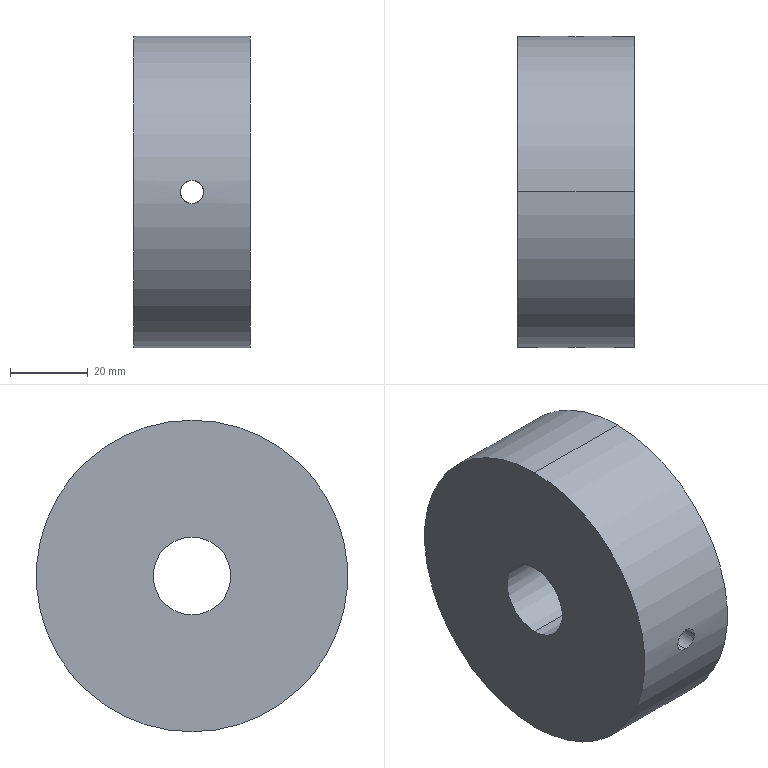Part | NX | features BREP 1 | 1 solid | 10 faces | box 30 x 80 x 80 mm | volume 139671 mm3 | cylinder 8 | plane 2 | commonest cylinder face diameters 6 x4 20 x2 80 x2
STEP:
#1=CARTESIAN_POINT('',(15.,39.887,-3.));
#2=VERTEX_POINT('',#1);
#3=CARTESIAN_POINT('',(15.,39.887,3.));
#4=VERTEX_POINT('',#3);
#5=CARTESIAN_POINT('',(15.,39.887,-3.));
#6=CARTESIAN_POINT('',(14.207,39.887,-3.));
#7=CARTESIAN_POINT('',(12.654,39.944,-2.35));
#8=CARTESIAN_POINT('',(11.674,40.028,-0.00292));
#9=CARTESIAN_POINT('',(12.651,39.944,2.349));
#10=CARTESIAN_POINT('',(14.207,39.887,3.));
#11=CARTESIAN_POINT('',(15.,39.887,3.));
#12=B_SPLINE_CURVE_WITH_KNOTS('',3,(#5,#6,#7,#8,#9,#10,#11),.UNSPECIFIED.,.F.,.F.,(4,1,1,1,4),(0.,0.002345,0.00469,0.007035,0.009381),.UNSPECIFIED.);
#13=EDGE_CURVE('',#2,#4,#12,.T.);
#14=ORIENTED_EDGE('',*,*,#13,.T.);
#15=CARTESIAN_POINT('',(15.,9.539,3.));
#16=VERTEX_POINT('',#15);
#17=CARTESIAN_POINT('',(15.,40.,3.));
#18=DIRECTION('',(0.,-1.,0.));
#19=VECTOR('',#18,1000.);
#20=LINE('',#17,#19);
#21=EDGE_CURVE('',#16,#4,#20,.F.);
#22=ORIENTED_EDGE('',*,*,#21,.F.);
#23=CARTESIAN_POINT('',(15.,9.539,-3.));
#24=VERTEX_POINT('',#23);
#25=CARTESIAN_POINT('',(15.,9.539,-3.));
#26=CARTESIAN_POINT('',(14.202,9.539,-3.));
#27=CARTESIAN_POINT('',(12.656,9.775,-2.35));
#28=CARTESIAN_POINT('',(11.672,10.112,-0.004774));
#29=CARTESIAN_POINT('',(12.655,9.775,2.351));
#30=CARTESIAN_POINT('',(14.202,9.539,3.));
#31=CARTESIAN_POINT('',(15.,9.539,3.));
#32=B_SPLINE_CURVE_WITH_KNOTS('',3,(#25,#26,#27,#28,#29,#30,#31),.UNSPECIFIED.,.F.,.F.,(4,1,1,1,4),(0.,0.002358,0.004715,0.007073,0.009431),.UNSPECIFIED.);
#33=EDGE_CURVE('',#24,#16,#32,.T.);
#34=ORIENTED_EDGE('',*,*,#33,.F.);
#35=CARTESIAN_POINT('',(15.,40.,-3.));
#36=DIRECTION('',(0.,-1.,0.));
#37=VECTOR('',#36,1000.);
#38=LINE('',#35,#37);
#39=EDGE_CURVE('',#24,#2,#38,.F.);
#40=ORIENTED_EDGE('',*,*,#39,.T.);
#41=EDGE_LOOP('',(#14,#22,#34,#40));
#42=FACE_BOUND('',#41,.T.);
#43=CARTESIAN_POINT('',(15.,40.,0.));
#44=DIRECTION('',(0.,-1.,0.));
#45=DIRECTION('',(0.,0.,1.));
#46=AXIS2_PLACEMENT_3D('',#43,#44,#45);
#47=CYLINDRICAL_SURFACE('',#46,3.);
#48=ADVANCED_FACE('',(#42),#47,.F.);
#49=CARTESIAN_POINT('',(15.,-9.539,3.));
#50=VERTEX_POINT('',#49);
#51=CARTESIAN_POINT('',(15.,-9.539,-3.));
#52=VERTEX_POINT('',#51);
#53=CARTESIAN_POINT('',(15.,-9.539,3.));
#54=CARTESIAN_POINT('',(14.202,-9.539,3.));
#55=CARTESIAN_POINT('',(12.656,-9.775,2.35));
#56=CARTESIAN_POINT('',(11.672,-10.112,0.004774));
#57=CARTESIAN_POINT('',(12.655,-9.775,-2.351));
#58=CARTESIAN_POINT('',(14.202,-9.539,-3.));
#59=CARTESIAN_POINT('',(15.,-9.539,-3.));
#60=B_SPLINE_CURVE_WITH_KNOTS('',3,(#53,#54,#55,#56,#57,#58,#59),.UNSPECIFIED.,.F.,.F.,(4,1,1,1,4),(0.,0.002358,0.004715,0.007073,0.009431),.UNSPECIFIED.);
#61=EDGE_CURVE('',#50,#52,#60,.T.);
#62=ORIENTED_EDGE('',*,*,#61,.F.);
#63=CARTESIAN_POINT('',(15.,-39.887,3.));
#64=VERTEX_POINT('',#63);
#65=CARTESIAN_POINT('',(15.,40.,3.));
#66=DIRECTION('',(0.,-1.,0.));
#67=VECTOR('',#66,1000.);
#68=LINE('',#65,#67);
#69=EDGE_CURVE('',#64,#50,#68,.F.);
#70=ORIENTED_EDGE('',*,*,#69,.F.);
#71=CARTESIAN_POINT('',(15.,-39.887,-3.));
#72=VERTEX_POINT('',#71);
#73=CARTESIAN_POINT('',(15.,-39.887,3.));
#74=CARTESIAN_POINT('',(14.207,-39.887,3.));
#75=CARTESIAN_POINT('',(12.654,-39.944,2.35));
#76=CARTESIAN_POINT('',(11.674,-40.028,0.00292));
#77=CARTESIAN_POINT('',(12.651,-39.944,-2.349));
#78=CARTESIAN_POINT('',(14.207,-39.887,-3.));
#79=CARTESIAN_POINT('',(15.,-39.887,-3.));
#80=B_SPLINE_CURVE_WITH_KNOTS('',3,(#73,#74,#75,#76,#77,#78,#79),.UNSPECIFIED.,.F.,.F.,(4,1,1,1,4),(0.,0.002345,0.00469,0.007035,0.009381),.UNSPECIFIED.);
#81=EDGE_CURVE('',#64,#72,#80,.T.);
#82=ORIENTED_EDGE('',*,*,#81,.T.);
#83=CARTESIAN_POINT('',(15.,40.,-3.));
#84=DIRECTION('',(0.,-1.,0.));
#85=VECTOR('',#84,1000.);
#86=LINE('',#83,#85);
#87=EDGE_CURVE('',#72,#52,#86,.F.);
#88=ORIENTED_EDGE('',*,*,#87,.T.);
#89=EDGE_LOOP('',(#62,#70,#82,#88));
#90=FACE_BOUND('',#89,.T.);
#91=CARTESIAN_POINT('',(15.,40.,0.));
#92=DIRECTION('',(0.,-1.,0.));
#93=DIRECTION('',(0.,0.,1.));
#94=AXIS2_PLACEMENT_3D('',#91,#92,#93);
#95=CYLINDRICAL_SURFACE('',#94,3.);
#96=ADVANCED_FACE('',(#90),#95,.F.);
#97=CARTESIAN_POINT('',(30.,0.,10.));
#98=VERTEX_POINT('',#97);
#99=CARTESIAN_POINT('',(30.,0.,-10.));
#100=VERTEX_POINT('',#99);
#101=CARTESIAN_POINT('',(30.,0.,0.));
#102=DIRECTION('',(1.,0.,0.));
#103=DIRECTION('',(0.,0.,-1.));
#104=AXIS2_PLACEMENT_3D('',#101,#102,#103);
#105=CIRCLE('',#104,10.);
#106=EDGE_CURVE('',#98,#100,#105,.T.);
#107=ORIENTED_EDGE('',*,*,#106,.T.);
#108=CARTESIAN_POINT('',(0.,0.,-10.));
#109=VERTEX_POINT('',#108);
#110=CARTESIAN_POINT('',(30.,0.,-10.));
#111=DIRECTION('',(-1.,0.,0.));
#112=VECTOR('',#111,1000.);
#113=LINE('',#110,#112);
#114=EDGE_CURVE('',#100,#109,#113,.T.);
#115=ORIENTED_EDGE('',*,*,#114,.T.);
#116=CARTESIAN_POINT('',(0.,0.,10.));
#117=VERTEX_POINT('',#116);
#118=CARTESIAN_POINT('',(0.,0.,0.));
#119=DIRECTION('',(1.,0.,0.));
#120=DIRECTION('',(0.,0.,-1.));
#121=AXIS2_PLACEMENT_3D('',#118,#119,#120);
#122=CIRCLE('',#121,10.);
#123=EDGE_CURVE('',#117,#109,#122,.T.);
#124=ORIENTED_EDGE('',*,*,#123,.F.);
#125=CARTESIAN_POINT('',(30.,0.,10.));
#126=DIRECTION('',(-1.,0.,0.));
#127=VECTOR('',#126,1000.);
#128=LINE('',#125,#127);
#129=EDGE_CURVE('',#98,#117,#128,.T.);
#130=ORIENTED_EDGE('',*,*,#129,.F.);
#131=EDGE_LOOP('',(#107,#115,#124,#130));
#132=FACE_BOUND('',#131,.T.);
#133=CARTESIAN_POINT('',(15.,-9.539,-3.));
#134=CARTESIAN_POINT('',(15.798,-9.539,-3.));
#135=CARTESIAN_POINT('',(17.344,-9.775,-2.35));
#136=CARTESIAN_POINT('',(18.328,-10.112,-0.004774));
#137=CARTESIAN_POINT('',(17.345,-9.775,2.351));
#138=CARTESIAN_POINT('',(15.798,-9.539,3.));
#139=CARTESIAN_POINT('',(15.,-9.539,3.));
#140=B_SPLINE_CURVE_WITH_KNOTS('',3,(#133,#134,#135,#136,#137,#138,#139),.UNSPECIFIED.,.F.,.F.,(4,1,1,1,4),(0.,0.002358,0.004715,0.007073,0.009431),.UNSPECIFIED.);
#141=EDGE_CURVE('',#52,#50,#140,.T.);
#142=ORIENTED_EDGE('',*,*,#141,.T.);
#143=ORIENTED_EDGE('',*,*,#61,.T.);
#144=EDGE_LOOP('',(#142,#143));
#145=FACE_BOUND('',#144,.T.);
#146=CARTESIAN_POINT('',(30.,0.,0.));
#147=DIRECTION('',(-1.,0.,0.));
#148=DIRECTION('',(0.,0.,-1.));
#149=AXIS2_PLACEMENT_3D('',#146,#147,#148);
#150=CYLINDRICAL_SURFACE('',#149,10.);
#151=ADVANCED_FACE('',(#132,#145),#150,.F.);
#152=CARTESIAN_POINT('',(30.,0.,-40.));
#153=VERTEX_POINT('',#152);
#154=CARTESIAN_POINT('',(30.,0.,40.));
#155=VERTEX_POINT('',#154);
#156=CARTESIAN_POINT('',(30.,0.,0.));
#157=DIRECTION('',(1.,0.,0.));
#158=DIRECTION('',(0.,0.,-1.));
#159=AXIS2_PLACEMENT_3D('',#156,#157,#158);
#160=CIRCLE('',#159,40.);
#161=EDGE_CURVE('',#153,#155,#160,.T.);
#162=ORIENTED_EDGE('',*,*,#161,.F.);
#163=CARTESIAN_POINT('',(0.,0.,-40.));
#164=VERTEX_POINT('',#163);
#165=CARTESIAN_POINT('',(30.,0.,-40.));
#166=DIRECTION('',(-1.,0.,0.));
#167=VECTOR('',#166,1000.);
#168=LINE('',#165,#167);
#169=EDGE_CURVE('',#153,#164,#168,.T.);
#170=ORIENTED_EDGE('',*,*,#169,.T.);
#171=CARTESIAN_POINT('',(0.,0.,40.));
#172=VERTEX_POINT('',#171);
#173=CARTESIAN_POINT('',(0.,0.,0.));
#174=DIRECTION('',(1.,0.,0.));
#175=DIRECTION('',(0.,0.,-1.));
#176=AXIS2_PLACEMENT_3D('',#173,#174,#175);
#177=CIRCLE('',#176,40.);
#178=EDGE_CURVE('',#164,#172,#177,.T.);
#179=ORIENTED_EDGE('',*,*,#178,.T.);
#180=CARTESIAN_POINT('',(30.,0.,40.));
#181=DIRECTION('',(-1.,0.,0.));
#182=VECTOR('',#181,1000.);
#183=LINE('',#180,#182);
#184=EDGE_CURVE('',#155,#172,#183,.T.);
#185=ORIENTED_EDGE('',*,*,#184,.F.);
#186=EDGE_LOOP('',(#162,#170,#179,#185));
#187=FACE_BOUND('',#186,.T.);
#188=ORIENTED_EDGE('',*,*,#13,.F.);
#189=CARTESIAN_POINT('',(15.,39.887,3.));
#190=CARTESIAN_POINT('',(15.793,39.887,3.));
#191=CARTESIAN_POINT('',(17.346,39.944,2.35));
#192=CARTESIAN_POINT('',(18.326,40.028,0.00292));
#193=CARTESIAN_POINT('',(17.349,39.944,-2.349));
#194=CARTESIAN_POINT('',(15.793,39.887,-3.));
#195=CARTESIAN_POINT('',(15.,39.887,-3.));
#196=B_SPLINE_CURVE_WITH_KNOTS('',3,(#189,#190,#191,#192,#193,#194,#195),.UNSPECIFIED.,.F.,.F.,(4,1,1,1,4),(0.,0.002345,0.00469,0.007035,0.009381),.UNSPECIFIED.);
#197=EDGE_CURVE('',#4,#2,#196,.T.);
#198=ORIENTED_EDGE('',*,*,#197,.F.);
#199=EDGE_LOOP('',(#188,#198));
#200=FACE_BOUND('',#199,.T.);
#201=CARTESIAN_POINT('',(30.,0.,0.));
#202=DIRECTION('',(-1.,0.,0.));
#203=DIRECTION('',(0.,0.,-1.));
#204=AXIS2_PLACEMENT_3D('',#201,#202,#203);
#205=CYLINDRICAL_SURFACE('',#204,40.);
#206=ADVANCED_FACE('',(#187,#200),#205,.T.);
#207=ORIENTED_EDGE('',*,*,#169,.F.);
#208=CARTESIAN_POINT('',(30.,0.,0.));
#209=DIRECTION('',(1.,0.,0.));
#210=DIRECTION('',(0.,0.,-1.));
#211=AXIS2_PLACEMENT_3D('',#208,#209,#210);
#212=CIRCLE('',#211,40.);
#213=EDGE_CURVE('',#155,#153,#212,.T.);
#214=ORIENTED_EDGE('',*,*,#213,.F.);
#215=ORIENTED_EDGE('',*,*,#184,.T.);
#216=CARTESIAN_POINT('',(0.,0.,0.));
#217=DIRECTION('',(1.,0.,0.));
#218=DIRECTION('',(0.,0.,-1.));
#219=AXIS2_PLACEMENT_3D('',#216,#217,#218);
#220=CIRCLE('',#219,40.);
#221=EDGE_CURVE('',#172,#164,#220,.T.);
#222=ORIENTED_EDGE('',*,*,#221,.T.);
#223=EDGE_LOOP('',(#207,#214,#215,#222));
#224=FACE_BOUND('',#223,.T.);
#225=CARTESIAN_POINT('',(15.,-39.887,-3.));
#226=CARTESIAN_POINT('',(15.793,-39.887,-3.));
#227=CARTESIAN_POINT('',(17.346,-39.944,-2.35));
#228=CARTESIAN_POINT('',(18.326,-40.028,-0.00292));
#229=CARTESIAN_POINT('',(17.349,-39.944,2.349));
#230=CARTESIAN_POINT('',(15.793,-39.887,3.));
#231=CARTESIAN_POINT('',(15.,-39.887,3.));
#232=B_SPLINE_CURVE_WITH_KNOTS('',3,(#225,#226,#227,#228,#229,#230,#231),.UNSPECIFIED.,.F.,.F.,(4,1,1,1,4),(0.,0.002345,0.00469,0.007035,0.009381),.UNSPECIFIED.);
#233=EDGE_CURVE('',#72,#64,#232,.T.);
#234=ORIENTED_EDGE('',*,*,#233,.F.);
#235=ORIENTED_EDGE('',*,*,#81,.F.);
#236=EDGE_LOOP('',(#234,#235));
#237=FACE_BOUND('',#236,.T.);
#238=CARTESIAN_POINT('',(30.,0.,0.));
#239=DIRECTION('',(-1.,0.,0.));
#240=DIRECTION('',(0.,0.,-1.));
#241=AXIS2_PLACEMENT_3D('',#238,#239,#240);
#242=CYLINDRICAL_SURFACE('',#241,40.);
#243=ADVANCED_FACE('',(#224,#237),#242,.T.);
#244=ORIENTED_EDGE('',*,*,#114,.F.);
#245=CARTESIAN_POINT('',(30.,0.,0.));
#246=DIRECTION('',(1.,0.,0.));
#247=DIRECTION('',(0.,0.,-1.));
#248=AXIS2_PLACEMENT_3D('',#245,#246,#247);
#249=CIRCLE('',#248,10.);
#250=EDGE_CURVE('',#100,#98,#249,.T.);
#251=ORIENTED_EDGE('',*,*,#250,.T.);
#252=ORIENTED_EDGE('',*,*,#129,.T.);
#253=CARTESIAN_POINT('',(0.,0.,0.));
#254=DIRECTION('',(1.,0.,0.));
#255=DIRECTION('',(0.,0.,-1.));
#256=AXIS2_PLACEMENT_3D('',#253,#254,#255);
#257=CIRCLE('',#256,10.);
#258=EDGE_CURVE('',#109,#117,#257,.T.);
#259=ORIENTED_EDGE('',*,*,#258,.F.);
#260=EDGE_LOOP('',(#244,#251,#252,#259));
#261=FACE_BOUND('',#260,.T.);
#262=ORIENTED_EDGE('',*,*,#33,.T.);
#263=CARTESIAN_POINT('',(15.,9.539,3.));
#264=CARTESIAN_POINT('',(15.798,9.539,3.));
#265=CARTESIAN_POINT('',(17.344,9.775,2.35));
#266=CARTESIAN_POINT('',(18.328,10.112,0.004774));
#267=CARTESIAN_POINT('',(17.345,9.775,-2.351));
#268=CARTESIAN_POINT('',(15.798,9.539,-3.));
#269=CARTESIAN_POINT('',(15.,9.539,-3.));
#270=B_SPLINE_CURVE_WITH_KNOTS('',3,(#263,#264,#265,#266,#267,#268,#269),.UNSPECIFIED.,.F.,.F.,(4,1,1,1,4),(0.,0.002358,0.004715,0.007073,0.009431),.UNSPECIFIED.);
#271=EDGE_CURVE('',#16,#24,#270,.T.);
#272=ORIENTED_EDGE('',*,*,#271,.T.);
#273=EDGE_LOOP('',(#262,#272));
#274=FACE_BOUND('',#273,.T.);
#275=CARTESIAN_POINT('',(30.,0.,0.));
#276=DIRECTION('',(-1.,0.,0.));
#277=DIRECTION('',(0.,0.,-1.));
#278=AXIS2_PLACEMENT_3D('',#275,#276,#277);
#279=CYLINDRICAL_SURFACE('',#278,10.);
#280=ADVANCED_FACE('',(#261,#274),#279,.F.);
#281=ORIENTED_EDGE('',*,*,#213,.T.);
#282=ORIENTED_EDGE('',*,*,#161,.T.);
#283=EDGE_LOOP('',(#281,#282));
#284=FACE_BOUND('',#283,.T.);
#285=ORIENTED_EDGE('',*,*,#106,.F.);
#286=ORIENTED_EDGE('',*,*,#250,.F.);
#287=EDGE_LOOP('',(#285,#286));
#288=FACE_BOUND('',#287,.T.);
#289=CARTESIAN_POINT('',(30.,0.,0.));
#290=DIRECTION('',(1.,0.,0.));
#291=DIRECTION('',(0.,0.,1.));
#292=AXIS2_PLACEMENT_3D('',#289,#290,#291);
#293=PLANE('',#292);
#294=ADVANCED_FACE('',(#284,#288),#293,.T.);
#295=ORIENTED_EDGE('',*,*,#221,.F.);
#296=ORIENTED_EDGE('',*,*,#178,.F.);
#297=EDGE_LOOP('',(#295,#296));
#298=FACE_BOUND('',#297,.T.);
#299=ORIENTED_EDGE('',*,*,#123,.T.);
#300=ORIENTED_EDGE('',*,*,#258,.T.);
#301=EDGE_LOOP('',(#299,#300));
#302=FACE_BOUND('',#301,.T.);
#303=CARTESIAN_POINT('',(0.,0.,0.));
#304=DIRECTION('',(1.,0.,0.));
#305=DIRECTION('',(0.,0.,1.));
#306=AXIS2_PLACEMENT_3D('',#303,#304,#305);
#307=PLANE('',#306);
#308=ADVANCED_FACE('',(#298,#302),#307,.F.);
#309=ORIENTED_EDGE('',*,*,#69,.T.);
#310=ORIENTED_EDGE('',*,*,#141,.F.);
#311=ORIENTED_EDGE('',*,*,#87,.F.);
#312=ORIENTED_EDGE('',*,*,#233,.T.);
#313=EDGE_LOOP('',(#309,#310,#311,#312));
#314=FACE_BOUND('',#313,.T.);
#315=CARTESIAN_POINT('',(15.,40.,0.));
#316=DIRECTION('',(0.,-1.,0.));
#317=DIRECTION('',(0.,0.,1.));
#318=AXIS2_PLACEMENT_3D('',#315,#316,#317);
#319=CYLINDRICAL_SURFACE('',#318,3.);
#320=ADVANCED_FACE('',(#314),#319,.F.);
#321=ORIENTED_EDGE('',*,*,#21,.T.);
#322=ORIENTED_EDGE('',*,*,#197,.T.);
#323=ORIENTED_EDGE('',*,*,#39,.F.);
#324=ORIENTED_EDGE('',*,*,#271,.F.);
#325=EDGE_LOOP('',(#321,#322,#323,#324));
#326=FACE_BOUND('',#325,.T.);
#327=CARTESIAN_POINT('',(15.,40.,0.));
#328=DIRECTION('',(0.,-1.,0.));
#329=DIRECTION('',(0.,0.,1.));
#330=AXIS2_PLACEMENT_3D('',#327,#328,#329);
#331=CYLINDRICAL_SURFACE('',#330,3.);
#332=ADVANCED_FACE('',(#326),#331,.F.);
#333=CLOSED_SHELL('',(#48,#96,#151,#206,#243,#280,#294,#308,#320,#332));
#334=MANIFOLD_SOLID_BREP('',#333);
#335=(LENGTH_UNIT()NAMED_UNIT(*)SI_UNIT(.MILLI.,.METRE.));
#336=UNCERTAINTY_MEASURE_WITH_UNIT(LENGTH_MEASURE(0.0508),#335,'','');
#337=(NAMED_UNIT(*)PLANE_ANGLE_UNIT()SI_UNIT($,.RADIAN.));
#338=(NAMED_UNIT(*)SI_UNIT($,.STERADIAN.)SOLID_ANGLE_UNIT());
#339=(GEOMETRIC_REPRESENTATION_CONTEXT(3)GLOBAL_UNCERTAINTY_ASSIGNED_CONTEXT((#336))GLOBAL_UNIT_ASSIGNED_CONTEXT((#335,#337,#338))REPRESENTATION_CONTEXT('',''));
#340=ADVANCED_BREP_SHAPE_REPRESENTATION('',(#334),#339);